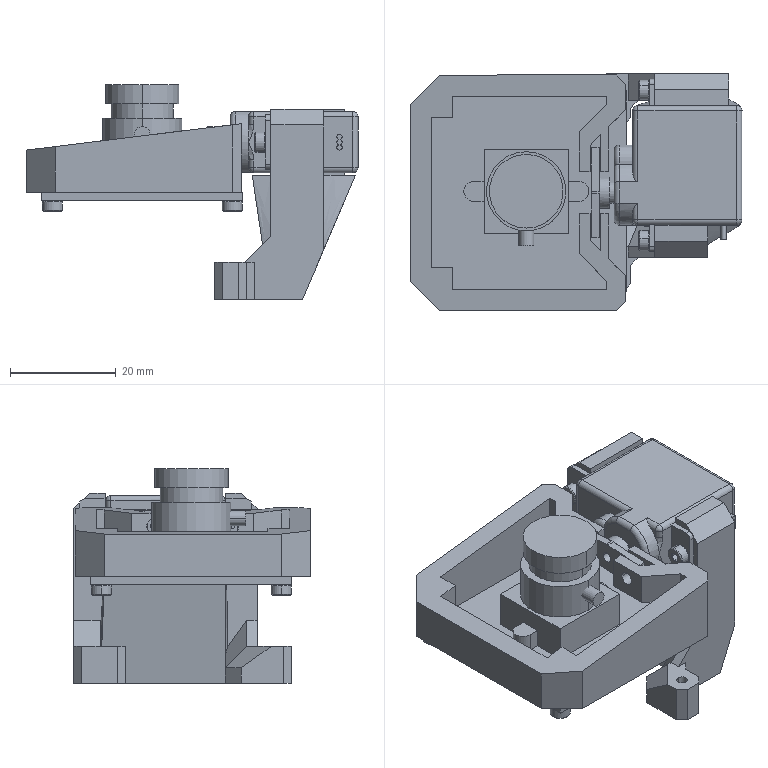Part | SolidWorks | features BaseBody 12 | 12 solids | 895 faces | box 62.8 x 44.75 x 40.65 mm | volume 30642 mm3 | cylinder 579 | plane 207 | cone 78 | spline 18 | sphere 8 | torus 5 | commonest cylinder face diameters 2 x269 1.48 x240 3.8 x14 1 x13 2.5 x12 2.2 x8